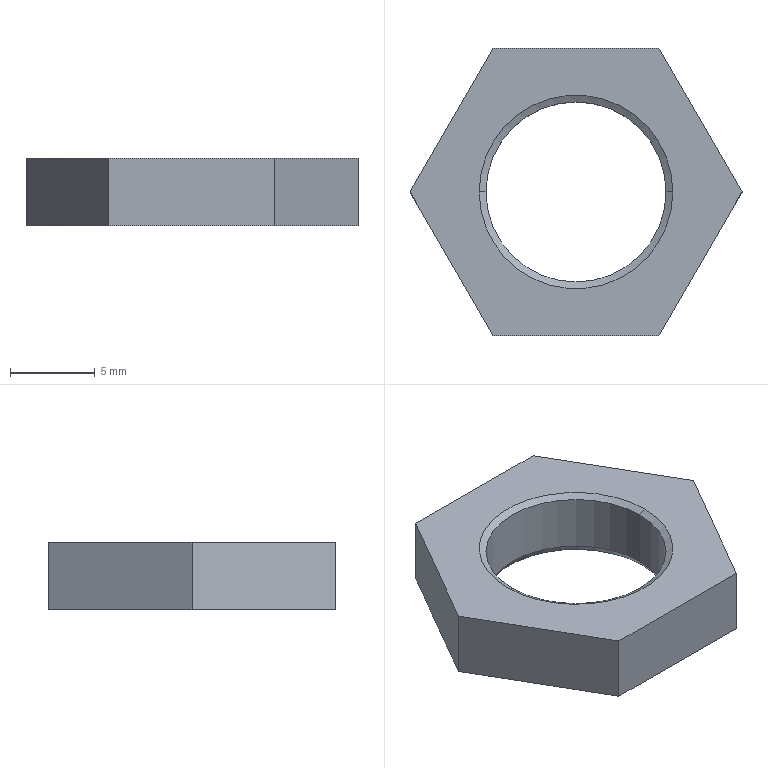Part | STEP file | Fine-Thread Nut M12X1_GB_FASTENER_NUT_STNABTT M12X1.25-N | 1 solid | 14 faces | box 19.63 x 17 x 4 mm | volume 641.848 mm3 | plane 8 | cone 4 | cylinder 2 | commonest cylinder face diameters 10.647 x2
STEP:
#1=CARTESIAN_POINT('',(0.,0.,0.));
#2=DIRECTION('',(0.,0.,1.));
#3=DIRECTION('',(1.,0.,0.));
#4=AXIS2_PLACEMENT_3D('',#1,#2,#3);
#5=CARTESIAN_POINT('',(5.324,0.,-0.2309));
#6=VERTEX_POINT('',#5);
#7=CARTESIAN_POINT('',(5.723,0.,0.));
#8=VERTEX_POINT('',#7);
#9=CARTESIAN_POINT('',(5.324,0.,-0.2309));
#10=DIRECTION('',(0.866,0.,0.5));
#11=VECTOR('',#10,1.);
#12=LINE('',#9,#11);
#13=CARTESIAN_POINT('',(0.,0.,-0.2309));
#14=DIRECTION('',(0.,0.,1.));
#15=DIRECTION('',(1.,0.,0.));
#16=AXIS2_PLACEMENT_3D('',#13,#14,#15);
#17=CONICAL_SURFACE('',#16,5.324,1.047);
#18=CARTESIAN_POINT('',(6.283,0.));
#19=DIRECTION('',(0.,1.));
#20=VECTOR('',#19,1.);
#21=LINE('',#18,#20);
#22=(GEOMETRIC_REPRESENTATION_CONTEXT(2)PARAMETRIC_REPRESENTATION_CONTEXT()REPRESENTATION_CONTEXT('',''));
#23=DEFINITIONAL_REPRESENTATION('',(#21),#22);
#24=PCURVE('',#17,#23);
#25=CARTESIAN_POINT('',(0.,0.,-0.2309));
#26=DIRECTION('',(0.,0.,1.));
#27=DIRECTION('',(1.,0.,0.));
#28=AXIS2_PLACEMENT_3D('',#25,#26,#27);
#29=CONICAL_SURFACE('',#28,5.324,1.047);
#30=CARTESIAN_POINT('',(0.,0.));
#31=DIRECTION('',(0.,1.));
#32=VECTOR('',#31,1.);
#33=LINE('',#30,#32);
#34=(GEOMETRIC_REPRESENTATION_CONTEXT(2)PARAMETRIC_REPRESENTATION_CONTEXT()REPRESENTATION_CONTEXT('',''));
#35=DEFINITIONAL_REPRESENTATION('',(#33),#34);
#36=PCURVE('',#29,#35);
#37=SURFACE_CURVE('',#12,(#24,#36),.PCURVE_S1.);
#38=EDGE_CURVE('',#6,#8,#37,.T.);
#39=ORIENTED_EDGE('',*,*,#38,.T.);
#40=CARTESIAN_POINT('',(-5.723,0.,0.));
#41=VERTEX_POINT('',#40);
#42=CARTESIAN_POINT('',(0.,0.,0.));
#43=DIRECTION('',(0.,0.,-1.));
#44=DIRECTION('',(1.,0.,0.));
#45=AXIS2_PLACEMENT_3D('',#42,#43,#44);
#46=CIRCLE('',#45,5.723);
#47=CARTESIAN_POINT('',(6.283,0.2309));
#48=DIRECTION('',(-1.,0.));
#49=VECTOR('',#48,1.);
#50=LINE('',#47,#49);
#51=(GEOMETRIC_REPRESENTATION_CONTEXT(2)PARAMETRIC_REPRESENTATION_CONTEXT()REPRESENTATION_CONTEXT('',''));
#52=DEFINITIONAL_REPRESENTATION('',(#50),#51);
#53=PCURVE('',#17,#52);
#54=CARTESIAN_POINT('',(4.907,-8.5,0.));
#55=DIRECTION('',(0.,0.,1.));
#56=DIRECTION('',(1.,0.,0.));
#57=AXIS2_PLACEMENT_3D('',#54,#55,#56);
#58=PLANE('',#57);
#59=CARTESIAN_POINT('',(0.816,8.5));
#60=CARTESIAN_POINT('',(0.816,-1.413));
#61=CARTESIAN_POINT('',(-7.769,3.543));
#62=CARTESIAN_POINT('',(-16.354,8.5));
#63=CARTESIAN_POINT('',(-7.769,13.457));
#64=CARTESIAN_POINT('',(0.816,18.413));
#65=CARTESIAN_POINT('',(0.816,8.5));
#66=(BOUNDED_CURVE()B_SPLINE_CURVE(2,(#59,#60,#61,#62,#63,#64,#65),.UNSPECIFIED.,.T.,.F.)B_SPLINE_CURVE_WITH_KNOTS((1,2,2,2,2,1),(-2.094,0.,2.094,4.189,6.283,8.378),.UNSPECIFIED.)CURVE()GEOMETRIC_REPRESENTATION_ITEM()RATIONAL_B_SPLINE_CURVE((1.,0.5,1.,0.5,1.,0.5,1.))REPRESENTATION_ITEM(''));
#67=(GEOMETRIC_REPRESENTATION_CONTEXT(2)PARAMETRIC_REPRESENTATION_CONTEXT()REPRESENTATION_CONTEXT('',''));
#68=DEFINITIONAL_REPRESENTATION('',(#66),#67);
#69=PCURVE('',#58,#68);
#70=SURFACE_CURVE('',#46,(#53,#69),.PCURVE_S1.);
#71=EDGE_CURVE('',#8,#41,#70,.T.);
#72=ORIENTED_EDGE('',*,*,#71,.T.);
#73=CARTESIAN_POINT('',(-5.324,0.,-0.2309));
#74=VERTEX_POINT('',#73);
#75=CARTESIAN_POINT('',(-5.324,0.,-0.2309));
#76=DIRECTION('',(-0.866,0.,0.5));
#77=VECTOR('',#76,1.);
#78=LINE('',#75,#77);
#79=CARTESIAN_POINT('',(3.142,0.));
#80=DIRECTION('',(0.,1.));
#81=VECTOR('',#80,1.);
#82=LINE('',#79,#81);
#83=(GEOMETRIC_REPRESENTATION_CONTEXT(2)PARAMETRIC_REPRESENTATION_CONTEXT()REPRESENTATION_CONTEXT('',''));
#84=DEFINITIONAL_REPRESENTATION('',(#82),#83);
#85=PCURVE('',#17,#84);
#86=CARTESIAN_POINT('',(3.142,0.));
#87=DIRECTION('',(0.,1.));
#88=VECTOR('',#87,1.);
#89=LINE('',#86,#88);
#90=(GEOMETRIC_REPRESENTATION_CONTEXT(2)PARAMETRIC_REPRESENTATION_CONTEXT()REPRESENTATION_CONTEXT('',''));
#91=DEFINITIONAL_REPRESENTATION('',(#89),#90);
#92=PCURVE('',#29,#91);
#93=SURFACE_CURVE('',#78,(#85,#92),.PCURVE_S1.);
#94=EDGE_CURVE('',#74,#41,#93,.T.);
#95=ORIENTED_EDGE('',*,*,#94,.F.);
#96=CARTESIAN_POINT('',(0.,0.,-0.2309));
#97=DIRECTION('',(0.,0.,1.));
#98=DIRECTION('',(1.,0.,0.));
#99=AXIS2_PLACEMENT_3D('',#96,#97,#98);
#100=CIRCLE('',#99,5.324);
#101=CARTESIAN_POINT('',(0.,0.));
#102=DIRECTION('',(1.,0.));
#103=VECTOR('',#102,1.);
#104=LINE('',#101,#103);
#105=(GEOMETRIC_REPRESENTATION_CONTEXT(2)PARAMETRIC_REPRESENTATION_CONTEXT()REPRESENTATION_CONTEXT('',''));
#106=DEFINITIONAL_REPRESENTATION('',(#104),#105);
#107=PCURVE('',#17,#106);
#108=CARTESIAN_POINT('',(0.,0.,-4.));
#109=DIRECTION('',(0.,0.,1.));
#110=DIRECTION('',(1.,0.,0.));
#111=AXIS2_PLACEMENT_3D('',#108,#109,#110);
#112=CYLINDRICAL_SURFACE('',#111,5.324);
#113=CARTESIAN_POINT('',(0.,3.769));
#114=DIRECTION('',(1.,0.));
#115=VECTOR('',#114,1.);
#116=LINE('',#113,#115);
#117=(GEOMETRIC_REPRESENTATION_CONTEXT(2)PARAMETRIC_REPRESENTATION_CONTEXT()REPRESENTATION_CONTEXT('',''));
#118=DEFINITIONAL_REPRESENTATION('',(#116),#117);
#119=PCURVE('',#112,#118);
#120=SURFACE_CURVE('',#100,(#107,#119),.PCURVE_S1.);
#121=EDGE_CURVE('',#74,#6,#120,.T.);
#122=ORIENTED_EDGE('',*,*,#121,.T.);
#123=EDGE_LOOP('',(#39,#72,#95,#122));
#124=FACE_BOUND('',#123,.F.);
#125=ADVANCED_FACE('',(#124),#17,.F.);
#126=CARTESIAN_POINT('',(-5.324,0.,-3.6));
#127=VERTEX_POINT('',#126);
#128=CARTESIAN_POINT('',(-5.554,0.,-4.));
#129=VERTEX_POINT('',#128);
#130=CARTESIAN_POINT('',(-5.554,0.,-4.));
#131=DIRECTION('',(-0.5,0.,-0.866));
#132=VECTOR('',#131,1.);
#133=LINE('',#130,#132);
#134=CARTESIAN_POINT('',(0.,0.,-4.));
#135=DIRECTION('',(0.,0.,-1.));
#136=DIRECTION('',(-1.,0.,0.));
#137=AXIS2_PLACEMENT_3D('',#134,#135,#136);
#138=CONICAL_SURFACE('',#137,5.554,0.5236);
#139=CARTESIAN_POINT('',(6.283,0.));
#140=DIRECTION('',(0.,1.));
#141=VECTOR('',#140,1.);
#142=LINE('',#139,#141);
#143=(GEOMETRIC_REPRESENTATION_CONTEXT(2)PARAMETRIC_REPRESENTATION_CONTEXT()REPRESENTATION_CONTEXT('',''));
#144=DEFINITIONAL_REPRESENTATION('',(#142),#143);
#145=PCURVE('',#138,#144);
#146=CARTESIAN_POINT('',(0.,0.,-4.));
#147=DIRECTION('',(0.,0.,-1.));
#148=DIRECTION('',(-1.,0.,0.));
#149=AXIS2_PLACEMENT_3D('',#146,#147,#148);
#150=CONICAL_SURFACE('',#149,5.554,0.5236);
#151=CARTESIAN_POINT('',(0.,0.));
#152=DIRECTION('',(0.,1.));
#153=VECTOR('',#152,1.);
#154=LINE('',#151,#153);
#155=(GEOMETRIC_REPRESENTATION_CONTEXT(2)PARAMETRIC_REPRESENTATION_CONTEXT()REPRESENTATION_CONTEXT('',''));
#156=DEFINITIONAL_REPRESENTATION('',(#154),#155);
#157=PCURVE('',#150,#156);
#158=SURFACE_CURVE('',#133,(#145,#157),.PCURVE_S1.);
#159=EDGE_CURVE('',#127,#129,#158,.T.);
#160=ORIENTED_EDGE('',*,*,#159,.T.);
#161=CARTESIAN_POINT('',(5.554,0.,-4.));
#162=VERTEX_POINT('',#161);
#163=CARTESIAN_POINT('',(0.,0.,-4.));
#164=DIRECTION('',(0.,0.,1.));
#165=DIRECTION('',(1.,0.,0.));
#166=AXIS2_PLACEMENT_3D('',#163,#164,#165);
#167=CIRCLE('',#166,5.554);
#168=CARTESIAN_POINT('',(9.425,0.));
#169=DIRECTION('',(-1.,0.));
#170=VECTOR('',#169,1.);
#171=LINE('',#168,#170);
#172=(GEOMETRIC_REPRESENTATION_CONTEXT(2)PARAMETRIC_REPRESENTATION_CONTEXT()REPRESENTATION_CONTEXT('',''));
#173=DEFINITIONAL_REPRESENTATION('',(#171),#172);
#174=PCURVE('',#138,#173);
#175=CARTESIAN_POINT('',(4.907,-8.5,-4.));
#176=DIRECTION('',(0.,0.,1.));
#177=DIRECTION('',(1.,0.,0.));
#178=AXIS2_PLACEMENT_3D('',#175,#176,#177);
#179=PLANE('',#178);
#180=CARTESIAN_POINT('',(-4.907,8.5));
#181=DIRECTION('',(1.,0.));
#182=AXIS2_PLACEMENT_2D('',#180,#181);
#183=CIRCLE('',#182,5.554);
#184=(GEOMETRIC_REPRESENTATION_CONTEXT(2)PARAMETRIC_REPRESENTATION_CONTEXT()REPRESENTATION_CONTEXT('',''));
#185=DEFINITIONAL_REPRESENTATION('',(#183),#184);
#186=PCURVE('',#179,#185);
#187=SURFACE_CURVE('',#167,(#174,#186),.PCURVE_S1.);
#188=EDGE_CURVE('',#129,#162,#187,.T.);
#189=ORIENTED_EDGE('',*,*,#188,.T.);
#190=CARTESIAN_POINT('',(5.324,0.,-3.6));
#191=VERTEX_POINT('',#190);
#192=CARTESIAN_POINT('',(5.554,0.,-4.));
#193=DIRECTION('',(0.5,0.,-0.866));
#194=VECTOR('',#193,1.);
#195=LINE('',#192,#194);
#196=CARTESIAN_POINT('',(3.142,0.));
#197=DIRECTION('',(0.,1.));
#198=VECTOR('',#197,1.);
#199=LINE('',#196,#198);
#200=(GEOMETRIC_REPRESENTATION_CONTEXT(2)PARAMETRIC_REPRESENTATION_CONTEXT()REPRESENTATION_CONTEXT('',''));
#201=DEFINITIONAL_REPRESENTATION('',(#199),#200);
#202=PCURVE('',#138,#201);
#203=CARTESIAN_POINT('',(3.142,0.));
#204=DIRECTION('',(0.,1.));
#205=VECTOR('',#204,1.);
#206=LINE('',#203,#205);
#207=(GEOMETRIC_REPRESENTATION_CONTEXT(2)PARAMETRIC_REPRESENTATION_CONTEXT()REPRESENTATION_CONTEXT('',''));
#208=DEFINITIONAL_REPRESENTATION('',(#206),#207);
#209=PCURVE('',#150,#208);
#210=SURFACE_CURVE('',#195,(#202,#209),.PCURVE_S1.);
#211=EDGE_CURVE('',#191,#162,#210,.T.);
#212=ORIENTED_EDGE('',*,*,#211,.F.);
#213=CARTESIAN_POINT('',(0.,0.,-3.6));
#214=DIRECTION('',(0.,0.,-1.));
#215=DIRECTION('',(1.,0.,0.));
#216=AXIS2_PLACEMENT_3D('',#213,#214,#215);
#217=CIRCLE('',#216,5.324);
#218=CARTESIAN_POINT('',(3.142,-0.4));
#219=DIRECTION('',(1.,0.));
#220=VECTOR('',#219,1.);
#221=LINE('',#218,#220);
#222=(GEOMETRIC_REPRESENTATION_CONTEXT(2)PARAMETRIC_REPRESENTATION_CONTEXT()REPRESENTATION_CONTEXT('',''));
#223=DEFINITIONAL_REPRESENTATION('',(#221),#222);
#224=PCURVE('',#138,#223);
#225=CARTESIAN_POINT('',(6.283,0.4));
#226=DIRECTION('',(-1.,0.));
#227=VECTOR('',#226,1.);
#228=LINE('',#225,#227);
#229=(GEOMETRIC_REPRESENTATION_CONTEXT(2)PARAMETRIC_REPRESENTATION_CONTEXT()REPRESENTATION_CONTEXT('',''));
#230=DEFINITIONAL_REPRESENTATION('',(#228),#229);
#231=PCURVE('',#112,#230);
#232=SURFACE_CURVE('',#217,(#224,#231),.PCURVE_S1.);
#233=EDGE_CURVE('',#191,#127,#232,.T.);
#234=ORIENTED_EDGE('',*,*,#233,.T.);
#235=EDGE_LOOP('',(#160,#189,#212,#234));
#236=FACE_BOUND('',#235,.F.);
#237=ADVANCED_FACE('',(#236),#138,.F.);
#238=CARTESIAN_POINT('',(5.324,0.,-4.));
#239=DIRECTION('',(0.,0.,1.));
#240=VECTOR('',#239,1.);
#241=LINE('',#238,#240);
#242=CARTESIAN_POINT('',(6.283,0.));
#243=DIRECTION('',(0.,1.));
#244=VECTOR('',#243,1.);
#245=LINE('',#242,#244);
#246=(GEOMETRIC_REPRESENTATION_CONTEXT(2)PARAMETRIC_REPRESENTATION_CONTEXT()REPRESENTATION_CONTEXT('',''));
#247=DEFINITIONAL_REPRESENTATION('',(#245),#246);
#248=PCURVE('',#112,#247);
#249=CARTESIAN_POINT('',(0.,0.,-4.));
#250=DIRECTION('',(0.,0.,1.));
#251=DIRECTION('',(1.,0.,0.));
#252=AXIS2_PLACEMENT_3D('',#249,#250,#251);
#253=CYLINDRICAL_SURFACE('',#252,5.324);
#254=CARTESIAN_POINT('',(0.,0.));
#255=DIRECTION('',(0.,1.));
#256=VECTOR('',#255,1.);
#257=LINE('',#254,#256);
#258=(GEOMETRIC_REPRESENTATION_CONTEXT(2)PARAMETRIC_REPRESENTATION_CONTEXT()REPRESENTATION_CONTEXT('',''));
#259=DEFINITIONAL_REPRESENTATION('',(#257),#258);
#260=PCURVE('',#253,#259);
#261=SURFACE_CURVE('',#241,(#248,#260),.PCURVE_S1.);
#262=EDGE_CURVE('',#191,#6,#261,.T.);
#263=ORIENTED_EDGE('',*,*,#262,.T.);
#264=ORIENTED_EDGE('',*,*,#121,.F.);
#265=CARTESIAN_POINT('',(-5.324,0.,-4.));
#266=DIRECTION('',(0.,0.,1.));
#267=VECTOR('',#266,1.);
#268=LINE('',#265,#267);
#269=CARTESIAN_POINT('',(3.142,0.));
#270=DIRECTION('',(0.,1.));
#271=VECTOR('',#270,1.);
#272=LINE('',#269,#271);
#273=(GEOMETRIC_REPRESENTATION_CONTEXT(2)PARAMETRIC_REPRESENTATION_CONTEXT()REPRESENTATION_CONTEXT('',''));
#274=DEFINITIONAL_REPRESENTATION('',(#272),#273);
#275=PCURVE('',#112,#274);
#276=CARTESIAN_POINT('',(3.142,0.));
#277=DIRECTION('',(0.,1.));
#278=VECTOR('',#277,1.);
#279=LINE('',#276,#278);
#280=(GEOMETRIC_REPRESENTATION_CONTEXT(2)PARAMETRIC_REPRESENTATION_CONTEXT()REPRESENTATION_CONTEXT('',''));
#281=DEFINITIONAL_REPRESENTATION('',(#279),#280);
#282=PCURVE('',#253,#281);
#283=SURFACE_CURVE('',#268,(#275,#282),.PCURVE_S1.);
#284=EDGE_CURVE('',#127,#74,#283,.T.);
#285=ORIENTED_EDGE('',*,*,#284,.F.);
#286=ORIENTED_EDGE('',*,*,#233,.F.);
#287=EDGE_LOOP('',(#263,#264,#285,#286));
#288=FACE_BOUND('',#287,.F.);
#289=ADVANCED_FACE('',(#288),#112,.F.);
#290=CARTESIAN_POINT('',(-4.907,-8.5,0.));
#291=VERTEX_POINT('',#290);
#292=CARTESIAN_POINT('',(4.907,-8.5,0.));
#293=VERTEX_POINT('',#292);
#294=CARTESIAN_POINT('',(-4.907,-8.5,0.));
#295=DIRECTION('',(1.,0.,0.));
#296=VECTOR('',#295,1.);
#297=LINE('',#294,#296);
#298=CARTESIAN_POINT('',(-4.907,-8.5,-4.));
#299=DIRECTION('',(0.,-1.,0.));
#300=DIRECTION('',(1.,0.,0.));
#301=AXIS2_PLACEMENT_3D('',#298,#299,#300);
#302=PLANE('',#301);
#303=CARTESIAN_POINT('',(0.,4.));
#304=DIRECTION('',(1.,0.));
#305=VECTOR('',#304,1.);
#306=LINE('',#303,#305);
#307=(GEOMETRIC_REPRESENTATION_CONTEXT(2)PARAMETRIC_REPRESENTATION_CONTEXT()REPRESENTATION_CONTEXT('',''));
#308=DEFINITIONAL_REPRESENTATION('',(#306),#307);
#309=PCURVE('',#302,#308);
#310=CARTESIAN_POINT('',(-9.815,0.));
#311=DIRECTION('',(1.,0.));
#312=VECTOR('',#311,1.);
#313=LINE('',#310,#312);
#314=(GEOMETRIC_REPRESENTATION_CONTEXT(2)PARAMETRIC_REPRESENTATION_CONTEXT()REPRESENTATION_CONTEXT('',''));
#315=DEFINITIONAL_REPRESENTATION('',(#313),#314);
#316=PCURVE('',#58,#315);
#317=SURFACE_CURVE('',#297,(#309,#316),.PCURVE_S1.);
#318=EDGE_CURVE('',#291,#293,#317,.T.);
#319=ORIENTED_EDGE('',*,*,#318,.F.);
#320=CARTESIAN_POINT('',(-4.907,-8.5,-4.));
#321=VERTEX_POINT('',#320);
#322=CARTESIAN_POINT('',(-4.907,-8.5,-4.));
#323=DIRECTION('',(0.,0.,1.));
#324=VECTOR('',#323,1.);
#325=LINE('',#322,#324);
#326=CARTESIAN_POINT('',(0.,0.));
#327=DIRECTION('',(0.,1.));
#328=VECTOR('',#327,1.);
#329=LINE('',#326,#328);
#330=(GEOMETRIC_REPRESENTATION_CONTEXT(2)PARAMETRIC_REPRESENTATION_CONTEXT()REPRESENTATION_CONTEXT('',''));
#331=DEFINITIONAL_REPRESENTATION('',(#329),#330);
#332=PCURVE('',#302,#331);
#333=CARTESIAN_POINT('',(-9.815,0.,-4.));
#334=DIRECTION('',(-0.866,-0.5,0.));
#335=DIRECTION('',(0.5,-0.866,0.));
#336=AXIS2_PLACEMENT_3D('',#333,#334,#335);
#337=PLANE('',#336);
#338=CARTESIAN_POINT('',(9.815,0.));
#339=DIRECTION('',(0.,1.));
#340=VECTOR('',#339,1.);
#341=LINE('',#338,#340);
#342=(GEOMETRIC_REPRESENTATION_CONTEXT(2)PARAMETRIC_REPRESENTATION_CONTEXT()REPRESENTATION_CONTEXT('',''));
#343=DEFINITIONAL_REPRESENTATION('',(#341),#342);
#344=PCURVE('',#337,#343);
#345=SURFACE_CURVE('',#325,(#332,#344),.PCURVE_S1.);
#346=EDGE_CURVE('',#321,#291,#345,.T.);
#347=ORIENTED_EDGE('',*,*,#346,.F.);
#348=CARTESIAN_POINT('',(4.907,-8.5,-4.));
#349=VERTEX_POINT('',#348);
#350=CARTESIAN_POINT('',(-4.907,-8.5,-4.));
#351=DIRECTION('',(1.,0.,0.));
#352=VECTOR('',#351,1.);
#353=LINE('',#350,#352);
#354=CARTESIAN_POINT('',(0.,0.));
#355=DIRECTION('',(1.,0.));
#356=VECTOR('',#355,1.);
#357=LINE('',#354,#356);
#358=(GEOMETRIC_REPRESENTATION_CONTEXT(2)PARAMETRIC_REPRESENTATION_CONTEXT()REPRESENTATION_CONTEXT('',''));
#359=DEFINITIONAL_REPRESENTATION('',(#357),#358);
#360=PCURVE('',#302,#359);
#361=CARTESIAN_POINT('',(-9.815,0.));
#362=DIRECTION('',(1.,0.));
#363=VECTOR('',#362,1.);
#364=LINE('',#361,#363);
#365=(GEOMETRIC_REPRESENTATION_CONTEXT(2)PARAMETRIC_REPRESENTATION_CONTEXT()REPRESENTATION_CONTEXT('',''));
#366=DEFINITIONAL_REPRESENTATION('',(#364),#365);
#367=PCURVE('',#179,#366);
#368=SURFACE_CURVE('',#353,(#360,#367),.PCURVE_S1.);
#369=EDGE_CURVE('',#321,#349,#368,.T.);
#370=ORIENTED_EDGE('',*,*,#369,.T.);
#371=CARTESIAN_POINT('',(4.907,-8.5,-4.));
#372=DIRECTION('',(0.,0.,1.));
#373=VECTOR('',#372,1.);
#374=LINE('',#371,#373);
#375=CARTESIAN_POINT('',(9.815,0.));
#376=DIRECTION('',(0.,1.));
#377=VECTOR('',#376,1.);
#378=LINE('',#375,#377);
#379=(GEOMETRIC_REPRESENTATION_CONTEXT(2)PARAMETRIC_REPRESENTATION_CONTEXT()REPRESENTATION_CONTEXT('',''));
#380=DEFINITIONAL_REPRESENTATION('',(#378),#379);
#381=PCURVE('',#302,#380);
#382=CARTESIAN_POINT('',(4.907,-8.5,-4.));
#383=DIRECTION('',(0.866,-0.5,0.));
#384=DIRECTION('',(0.5,0.866,0.));
#385=AXIS2_PLACEMENT_3D('',#382,#383,#384);
#386=PLANE('',#385);
#387=CARTESIAN_POINT('',(0.,0.));
#388=DIRECTION('',(0.,1.));
#389=VECTOR('',#388,1.);
#390=LINE('',#387,#389);
#391=(GEOMETRIC_REPRESENTATION_CONTEXT(2)PARAMETRIC_REPRESENTATION_CONTEXT()REPRESENTATION_CONTEXT('',''));
#392=DEFINITIONAL_REPRESENTATION('',(#390),#391);
#393=PCURVE('',#386,#392);
#394=SURFACE_CURVE('',#374,(#381,#393),.PCURVE_S1.);
#395=EDGE_CURVE('',#349,#293,#394,.T.);
#396=ORIENTED_EDGE('',*,*,#395,.T.);
#397=EDGE_LOOP('',(#319,#347,#370,#396));
#398=FACE_BOUND('',#397,.T.);
#399=ADVANCED_FACE('',(#398),#302,.T.);
#400=CARTESIAN_POINT('',(-9.815,0.,0.));
#401=VERTEX_POINT('',#400);
#402=CARTESIAN_POINT('',(-9.815,0.,0.));
#403=DIRECTION('',(0.5,-0.866,0.));
#404=VECTOR('',#403,1.);
#405=LINE('',#402,#404);
#406=CARTESIAN_POINT('',(0.,4.));
#407=DIRECTION('',(1.,0.));
#408=VECTOR('',#407,1.);
#409=LINE('',#406,#408);
#410=(GEOMETRIC_REPRESENTATION_CONTEXT(2)PARAMETRIC_REPRESENTATION_CONTEXT()REPRESENTATION_CONTEXT('',''));
#411=DEFINITIONAL_REPRESENTATION('',(#409),#410);
#412=PCURVE('',#337,#411);
#413=CARTESIAN_POINT('',(-14.722,8.5));
#414=DIRECTION('',(0.5,-0.866));
#415=VECTOR('',#414,1.);
#416=LINE('',#413,#415);
#417=(GEOMETRIC_REPRESENTATION_CONTEXT(2)PARAMETRIC_REPRESENTATION_CONTEXT()REPRESENTATION_CONTEXT('',''));
#418=DEFINITIONAL_REPRESENTATION('',(#416),#417);
#419=PCURVE('',#58,#418);
#420=SURFACE_CURVE('',#405,(#412,#419),.PCURVE_S1.);
#421=EDGE_CURVE('',#401,#291,#420,.T.);
#422=ORIENTED_EDGE('',*,*,#421,.F.);
#423=CARTESIAN_POINT('',(-9.815,0.,-4.));
#424=VERTEX_POINT('',#423);
#425=CARTESIAN_POINT('',(-9.815,0.,-4.));
#426=DIRECTION('',(0.,0.,1.));
#427=VECTOR('',#426,1.);
#428=LINE('',#425,#427);
#429=CARTESIAN_POINT('',(0.,0.));
#430=DIRECTION('',(0.,1.));
#431=VECTOR('',#430,1.);
#432=LINE('',#429,#431);
#433=(GEOMETRIC_REPRESENTATION_CONTEXT(2)PARAMETRIC_REPRESENTATION_CONTEXT()REPRESENTATION_CONTEXT('',''));
#434=DEFINITIONAL_REPRESENTATION('',(#432),#433);
#435=PCURVE('',#337,#434);
#436=CARTESIAN_POINT('',(-4.907,8.5,-4.));
#437=DIRECTION('',(-0.866,0.5,0.));
#438=DIRECTION('',(-0.5,-0.866,0.));
#439=AXIS2_PLACEMENT_3D('',#436,#437,#438);
#440=PLANE('',#439);
#441=CARTESIAN_POINT('',(9.815,0.));
#442=DIRECTION('',(0.,1.));
#443=VECTOR('',#442,1.);
#444=LINE('',#441,#443);
#445=(GEOMETRIC_REPRESENTATION_CONTEXT(2)PARAMETRIC_REPRESENTATION_CONTEXT()REPRESENTATION_CONTEXT('',''));
#446=DEFINITIONAL_REPRESENTATION('',(#444),#445);
#447=PCURVE('',#440,#446);
#448=SURFACE_CURVE('',#428,(#435,#447),.PCURVE_S1.);
#449=EDGE_CURVE('',#424,#401,#448,.T.);
#450=ORIENTED_EDGE('',*,*,#449,.F.);
#451=CARTESIAN_POINT('',(-9.815,0.,-4.));
#452=DIRECTION('',(0.5,-0.866,0.));
#453=VECTOR('',#452,1.);
#454=LINE('',#451,#453);
#455=CARTESIAN_POINT('',(0.,0.));
#456=DIRECTION('',(1.,0.));
#457=VECTOR('',#456,1.);
#458=LINE('',#455,#457);
#459=(GEOMETRIC_REPRESENTATION_CONTEXT(2)PARAMETRIC_REPRESENTATION_CONTEXT()REPRESENTATION_CONTEXT('',''));
#460=DEFINITIONAL_REPRESENTATION('',(#458),#459);
#461=PCURVE('',#337,#460);
#462=CARTESIAN_POINT('',(-14.722,8.5));
#463=DIRECTION('',(0.5,-0.866));
#464=VECTOR('',#463,1.);
#465=LINE('',#462,#464);
#466=(GEOMETRIC_REPRESENTATION_CONTEXT(2)PARAMETRIC_REPRESENTATION_CONTEXT()REPRESENTATION_CONTEXT('',''));
#467=DEFINITIONAL_REPRESENTATION('',(#465),#466);
#468=PCURVE('',#179,#467);
#469=SURFACE_CURVE('',#454,(#461,#468),.PCURVE_S1.);
#470=EDGE_CURVE('',#424,#321,#469,.T.);
#471=ORIENTED_EDGE('',*,*,#470,.T.);
#472=ORIENTED_EDGE('',*,*,#346,.T.);
#473=EDGE_LOOP('',(#422,#450,#471,#472));
#474=FACE_BOUND('',#473,.T.);
#475=ADVANCED_FACE('',(#474),#337,.T.);
#476=CARTESIAN_POINT('',(-4.907,8.5,0.));
#477=VERTEX_POINT('',#476);
#478=CARTESIAN_POINT('',(-4.907,8.5,0.));
#479=DIRECTION('',(-0.5,-0.866,0.));
#480=VECTOR('',#479,1.);
#481=LINE('',#478,#480);
#482=CARTESIAN_POINT('',(0.,4.));
#483=DIRECTION('',(1.,0.));
#484=VECTOR('',#483,1.);
#485=LINE('',#482,#484);
#486=(GEOMETRIC_REPRESENTATION_CONTEXT(2)PARAMETRIC_REPRESENTATION_CONTEXT()REPRESENTATION_CONTEXT('',''));
#487=DEFINITIONAL_REPRESENTATION('',(#485),#486);
#488=PCURVE('',#440,#487);
#489=CARTESIAN_POINT('',(-9.815,17.));
#490=DIRECTION('',(-0.5,-0.866));
#491=VECTOR('',#490,1.);
#492=LINE('',#489,#491);
#493=(GEOMETRIC_REPRESENTATION_CONTEXT(2)PARAMETRIC_REPRESENTATION_CONTEXT()REPRESENTATION_CONTEXT('',''));
#494=DEFINITIONAL_REPRESENTATION('',(#492),#493);
#495=PCURVE('',#58,#494);
#496=SURFACE_CURVE('',#481,(#488,#495),.PCURVE_S1.);
#497=EDGE_CURVE('',#477,#401,#496,.T.);
#498=ORIENTED_EDGE('',*,*,#497,.F.);
#499=CARTESIAN_POINT('',(-4.907,8.5,-4.));
#500=VERTEX_POINT('',#499);
#501=CARTESIAN_POINT('',(-4.907,8.5,-4.));
#502=DIRECTION('',(0.,0.,1.));
#503=VECTOR('',#502,1.);
#504=LINE('',#501,#503);
#505=CARTESIAN_POINT('',(0.,0.));
#506=DIRECTION('',(0.,1.));
#507=VECTOR('',#506,1.);
#508=LINE('',#505,#507);
#509=(GEOMETRIC_REPRESENTATION_CONTEXT(2)PARAMETRIC_REPRESENTATION_CONTEXT()REPRESENTATION_CONTEXT('',''));
#510=DEFINITIONAL_REPRESENTATION('',(#508),#509);
#511=PCURVE('',#440,#510);
#512=CARTESIAN_POINT('',(4.907,8.5,-4.));
#513=DIRECTION('',(0.,1.,0.));
#514=DIRECTION('',(0.,0.,1.));
#515=AXIS2_PLACEMENT_3D('',#512,#513,#514);
#516=PLANE('',#515);
#517=CARTESIAN_POINT('',(0.,-9.815));
#518=DIRECTION('',(1.,0.));
#519=VECTOR('',#518,1.);
#520=LINE('',#517,#519);
#521=(GEOMETRIC_REPRESENTATION_CONTEXT(2)PARAMETRIC_REPRESENTATION_CONTEXT()REPRESENTATION_CONTEXT('',''));
#522=DEFINITIONAL_REPRESENTATION('',(#520),#521);
#523=PCURVE('',#516,#522);
#524=SURFACE_CURVE('',#504,(#511,#523),.PCURVE_S1.);
#525=EDGE_CURVE('',#500,#477,#524,.T.);
#526=ORIENTED_EDGE('',*,*,#525,.F.);
#527=CARTESIAN_POINT('',(-4.907,8.5,-4.));
#528=DIRECTION('',(-0.5,-0.866,0.));
#529=VECTOR('',#528,1.);
#530=LINE('',#527,#529);
#531=CARTESIAN_POINT('',(0.,0.));
#532=DIRECTION('',(1.,0.));
#533=VECTOR('',#532,1.);
#534=LINE('',#531,#533);
#535=(GEOMETRIC_REPRESENTATION_CONTEXT(2)PARAMETRIC_REPRESENTATION_CONTEXT()REPRESENTATION_CONTEXT('',''));
#536=DEFINITIONAL_REPRESENTATION('',(#534),#535);
#537=PCURVE('',#440,#536);
#538=CARTESIAN_POINT('',(-9.815,17.));
#539=DIRECTION('',(-0.5,-0.866));
#540=VECTOR('',#539,1.);
#541=LINE('',#538,#540);
#542=(GEOMETRIC_REPRESENTATION_CONTEXT(2)PARAMETRIC_REPRESENTATION_CONTEXT()REPRESENTATION_CONTEXT('',''));
#543=DEFINITIONAL_REPRESENTATION('',(#541),#542);
#544=PCURVE('',#179,#543);
#545=SURFACE_CURVE('',#530,(#537,#544),.PCURVE_S1.);
#546=EDGE_CURVE('',#500,#424,#545,.T.);
#547=ORIENTED_EDGE('',*,*,#546,.T.);
#548=ORIENTED_EDGE('',*,*,#449,.T.);
#549=EDGE_LOOP('',(#498,#526,#547,#548));
#550=FACE_BOUND('',#549,.T.);
#551=ADVANCED_FACE('',(#550),#440,.T.);
#552=CARTESIAN_POINT('',(4.907,8.5,0.));
#553=VERTEX_POINT('',#552);
#554=CARTESIAN_POINT('',(4.907,8.5,0.));
#555=DIRECTION('',(-1.,0.,0.));
#556=VECTOR('',#555,1.);
#557=LINE('',#554,#556);
#558=CARTESIAN_POINT('',(4.,0.));
#559=DIRECTION('',(0.,-1.));
#560=VECTOR('',#559,1.);
#561=LINE('',#558,#560);
#562=(GEOMETRIC_REPRESENTATION_CONTEXT(2)PARAMETRIC_REPRESENTATION_CONTEXT()REPRESENTATION_CONTEXT('',''));
#563=DEFINITIONAL_REPRESENTATION('',(#561),#562);
#564=PCURVE('',#516,#563);
#565=CARTESIAN_POINT('',(0.,17.));
#566=DIRECTION('',(-1.,0.));
#567=VECTOR('',#566,1.);
#568=LINE('',#565,#567);
#569=(GEOMETRIC_REPRESENTATION_CONTEXT(2)PARAMETRIC_REPRESENTATION_CONTEXT()REPRESENTATION_CONTEXT('',''));
#570=DEFINITIONAL_REPRESENTATION('',(#568),#569);
#571=PCURVE('',#58,#570);
#572=SURFACE_CURVE('',#557,(#564,#571),.PCURVE_S1.);
#573=EDGE_CURVE('',#553,#477,#572,.T.);
#574=ORIENTED_EDGE('',*,*,#573,.F.);
#575=CARTESIAN_POINT('',(4.907,8.5,-4.));
#576=VERTEX_POINT('',#575);
#577=CARTESIAN_POINT('',(4.907,8.5,-4.));
#578=DIRECTION('',(0.,0.,1.));
#579=VECTOR('',#578,1.);
#580=LINE('',#577,#579);
#581=CARTESIAN_POINT('',(0.,0.));
#582=DIRECTION('',(1.,0.));
#583=VECTOR('',#582,1.);
#584=LINE('',#581,#583);
#585=(GEOMETRIC_REPRESENTATION_CONTEXT(2)PARAMETRIC_REPRESENTATION_CONTEXT()REPRESENTATION_CONTEXT('',''));
#586=DEFINITIONAL_REPRESENTATION('',(#584),#585);
#587=PCURVE('',#516,#586);
#588=CARTESIAN_POINT('',(9.815,0.,-4.));
#589=DIRECTION('',(0.866,0.5,0.));
#590=DIRECTION('',(-0.5,0.866,0.));
#591=AXIS2_PLACEMENT_3D('',#588,#589,#590);
#592=PLANE('',#591);
#593=CARTESIAN_POINT('',(9.815,0.));
#594=DIRECTION('',(0.,1.));
#595=VECTOR('',#594,1.);
#596=LINE('',#593,#595);
#597=(GEOMETRIC_REPRESENTATION_CONTEXT(2)PARAMETRIC_REPRESENTATION_CONTEXT()REPRESENTATION_CONTEXT('',''));
#598=DEFINITIONAL_REPRESENTATION('',(#596),#597);
#599=PCURVE('',#592,#598);
#600=SURFACE_CURVE('',#580,(#587,#599),.PCURVE_S1.);
#601=EDGE_CURVE('',#576,#553,#600,.T.);
#602=ORIENTED_EDGE('',*,*,#601,.F.);
#603=CARTESIAN_POINT('',(4.907,8.5,-4.));
#604=DIRECTION('',(-1.,0.,0.));
#605=VECTOR('',#604,1.);
#606=LINE('',#603,#605);
#607=CARTESIAN_POINT('',(0.,0.));
#608=DIRECTION('',(0.,-1.));
#609=VECTOR('',#608,1.);
#610=LINE('',#607,#609);
#611=(GEOMETRIC_REPRESENTATION_CONTEXT(2)PARAMETRIC_REPRESENTATION_CONTEXT()REPRESENTATION_CONTEXT('',''));
#612=DEFINITIONAL_REPRESENTATION('',(#610),#611);
#613=PCURVE('',#516,#612);
#614=CARTESIAN_POINT('',(0.,17.));
#615=DIRECTION('',(-1.,0.));
#616=VECTOR('',#615,1.);
#617=LINE('',#614,#616);
#618=(GEOMETRIC_REPRESENTATION_CONTEXT(2)PARAMETRIC_REPRESENTATION_CONTEXT()REPRESENTATION_CONTEXT('',''));
#619=DEFINITIONAL_REPRESENTATION('',(#617),#618);
#620=PCURVE('',#179,#619);
#621=SURFACE_CURVE('',#606,(#613,#620),.PCURVE_S1.);
#622=EDGE_CURVE('',#576,#500,#621,.T.);
#623=ORIENTED_EDGE('',*,*,#622,.T.);
#624=ORIENTED_EDGE('',*,*,#525,.T.);
#625=EDGE_LOOP('',(#574,#602,#623,#624));
#626=FACE_BOUND('',#625,.T.);
#627=ADVANCED_FACE('',(#626),#516,.T.);
#628=CARTESIAN_POINT('',(9.815,0.,0.));
#629=VERTEX_POINT('',#628);
#630=CARTESIAN_POINT('',(9.815,0.,0.));
#631=DIRECTION('',(-0.5,0.866,0.));
#632=VECTOR('',#631,1.);
#633=LINE('',#630,#632);
#634=CARTESIAN_POINT('',(0.,4.));
#635=DIRECTION('',(1.,0.));
#636=VECTOR('',#635,1.);
#637=LINE('',#634,#636);
#638=(GEOMETRIC_REPRESENTATION_CONTEXT(2)PARAMETRIC_REPRESENTATION_CONTEXT()REPRESENTATION_CONTEXT('',''));
#639=DEFINITIONAL_REPRESENTATION('',(#637),#638);
#640=PCURVE('',#592,#639);
#641=CARTESIAN_POINT('',(4.907,8.5));
#642=DIRECTION('',(-0.5,0.866));
#643=VECTOR('',#642,1.);
#644=LINE('',#641,#643);
#645=(GEOMETRIC_REPRESENTATION_CONTEXT(2)PARAMETRIC_REPRESENTATION_CONTEXT()REPRESENTATION_CONTEXT('',''));
#646=DEFINITIONAL_REPRESENTATION('',(#644),#645);
#647=PCURVE('',#58,#646);
#648=SURFACE_CURVE('',#633,(#640,#647),.PCURVE_S1.);
#649=EDGE_CURVE('',#629,#553,#648,.T.);
#650=ORIENTED_EDGE('',*,*,#649,.F.);
#651=CARTESIAN_POINT('',(9.815,0.,-4.));
#652=VERTEX_POINT('',#651);
#653=CARTESIAN_POINT('',(9.815,0.,-4.));
#654=DIRECTION('',(0.,0.,1.));
#655=VECTOR('',#654,1.);
#656=LINE('',#653,#655);
#657=CARTESIAN_POINT('',(0.,0.));
#658=DIRECTION('',(0.,1.));
#659=VECTOR('',#658,1.);
#660=LINE('',#657,#659);
#661=(GEOMETRIC_REPRESENTATION_CONTEXT(2)PARAMETRIC_REPRESENTATION_CONTEXT()REPRESENTATION_CONTEXT('',''));
#662=DEFINITIONAL_REPRESENTATION('',(#660),#661);
#663=PCURVE('',#592,#662);
#664=CARTESIAN_POINT('',(9.815,0.));
#665=DIRECTION('',(0.,1.));
#666=VECTOR('',#665,1.);
#667=LINE('',#664,#666);
#668=(GEOMETRIC_REPRESENTATION_CONTEXT(2)PARAMETRIC_REPRESENTATION_CONTEXT()REPRESENTATION_CONTEXT('',''));
#669=DEFINITIONAL_REPRESENTATION('',(#667),#668);
#670=PCURVE('',#386,#669);
#671=SURFACE_CURVE('',#656,(#663,#670),.PCURVE_S1.);
#672=EDGE_CURVE('',#652,#629,#671,.T.);
#673=ORIENTED_EDGE('',*,*,#672,.F.);
#674=CARTESIAN_POINT('',(9.815,0.,-4.));
#675=DIRECTION('',(-0.5,0.866,0.));
#676=VECTOR('',#675,1.);
#677=LINE('',#674,#676);
#678=CARTESIAN_POINT('',(0.,0.));
#679=DIRECTION('',(1.,0.));
#680=VECTOR('',#679,1.);
#681=LINE('',#678,#680);
#682=(GEOMETRIC_REPRESENTATION_CONTEXT(2)PARAMETRIC_REPRESENTATION_CONTEXT()REPRESENTATION_CONTEXT('',''));
#683=DEFINITIONAL_REPRESENTATION('',(#681),#682);
#684=PCURVE('',#592,#683);
#685=CARTESIAN_POINT('',(4.907,8.5));
#686=DIRECTION('',(-0.5,0.866));
#687=VECTOR('',#686,1.);
#688=LINE('',#685,#687);
#689=(GEOMETRIC_REPRESENTATION_CONTEXT(2)PARAMETRIC_REPRESENTATION_CONTEXT()REPRESENTATION_CONTEXT('',''));
#690=DEFINITIONAL_REPRESENTATION('',(#688),#689);
#691=PCURVE('',#179,#690);
#692=SURFACE_CURVE('',#677,(#684,#691),.PCURVE_S1.);
#693=EDGE_CURVE('',#652,#576,#692,.T.);
#694=ORIENTED_EDGE('',*,*,#693,.T.);
#695=ORIENTED_EDGE('',*,*,#601,.T.);
#696=EDGE_LOOP('',(#650,#673,#694,#695));
#697=FACE_BOUND('',#696,.T.);
#698=ADVANCED_FACE('',(#697),#592,.T.);
#699=CARTESIAN_POINT('',(4.907,-8.5,0.));
#700=DIRECTION('',(0.5,0.866,0.));
#701=VECTOR('',#700,1.);
#702=LINE('',#699,#701);
#703=CARTESIAN_POINT('',(0.,4.));
#704=DIRECTION('',(1.,0.));
#705=VECTOR('',#704,1.);
#706=LINE('',#703,#705);
#707=(GEOMETRIC_REPRESENTATION_CONTEXT(2)PARAMETRIC_REPRESENTATION_CONTEXT()REPRESENTATION_CONTEXT('',''));
#708=DEFINITIONAL_REPRESENTATION('',(#706),#707);
#709=PCURVE('',#386,#708);
#710=CARTESIAN_POINT('',(0.,0.));
#711=DIRECTION('',(0.5,0.866));
#712=VECTOR('',#711,1.);
#713=LINE('',#710,#712);
#714=(GEOMETRIC_REPRESENTATION_CONTEXT(2)PARAMETRIC_REPRESENTATION_CONTEXT()REPRESENTATION_CONTEXT('',''));
#715=DEFINITIONAL_REPRESENTATION('',(#713),#714);
#716=PCURVE('',#58,#715);
#717=SURFACE_CURVE('',#702,(#709,#716),.PCURVE_S1.);
#718=EDGE_CURVE('',#293,#629,#717,.T.);
#719=ORIENTED_EDGE('',*,*,#718,.F.);
#720=ORIENTED_EDGE('',*,*,#395,.F.);
#721=CARTESIAN_POINT('',(4.907,-8.5,-4.));
#722=DIRECTION('',(0.5,0.866,0.));
#723=VECTOR('',#722,1.);
#724=LINE('',#721,#723);
#725=CARTESIAN_POINT('',(0.,0.));
#726=DIRECTION('',(1.,0.));
#727=VECTOR('',#726,1.);
#728=LINE('',#725,#727);
#729=(GEOMETRIC_REPRESENTATION_CONTEXT(2)PARAMETRIC_REPRESENTATION_CONTEXT()REPRESENTATION_CONTEXT('',''));
#730=DEFINITIONAL_REPRESENTATION('',(#728),#729);
#731=PCURVE('',#386,#730);
#732=CARTESIAN_POINT('',(0.,0.));
#733=DIRECTION('',(0.5,0.866));
#734=VECTOR('',#733,1.);
#735=LINE('',#732,#734);
#736=(GEOMETRIC_REPRESENTATION_CONTEXT(2)PARAMETRIC_REPRESENTATION_CONTEXT()REPRESENTATION_CONTEXT('',''));
#737=DEFINITIONAL_REPRESENTATION('',(#735),#736);
#738=PCURVE('',#179,#737);
#739=SURFACE_CURVE('',#724,(#731,#738),.PCURVE_S1.);
#740=EDGE_CURVE('',#349,#652,#739,.T.);
#741=ORIENTED_EDGE('',*,*,#740,.T.);
#742=ORIENTED_EDGE('',*,*,#672,.T.);
#743=EDGE_LOOP('',(#719,#720,#741,#742));
#744=FACE_BOUND('',#743,.T.);
#745=ADVANCED_FACE('',(#744),#386,.T.);
#746=ORIENTED_EDGE('',*,*,#188,.T.);
#747=CARTESIAN_POINT('',(0.,0.,-4.));
#748=DIRECTION('',(0.,0.,1.));
#749=DIRECTION('',(1.,0.,0.));
#750=AXIS2_PLACEMENT_3D('',#747,#748,#749);
#751=CIRCLE('',#750,5.554);
#752=CARTESIAN_POINT('',(-4.907,8.5));
#753=DIRECTION('',(1.,0.));
#754=AXIS2_PLACEMENT_2D('',#752,#753);
#755=CIRCLE('',#754,5.554);
#756=(GEOMETRIC_REPRESENTATION_CONTEXT(2)PARAMETRIC_REPRESENTATION_CONTEXT()REPRESENTATION_CONTEXT('',''));
#757=DEFINITIONAL_REPRESENTATION('',(#755),#756);
#758=PCURVE('',#179,#757);
#759=CARTESIAN_POINT('',(3.142,0.));
#760=DIRECTION('',(-1.,0.));
#761=VECTOR('',#760,1.);
#762=LINE('',#759,#761);
#763=(GEOMETRIC_REPRESENTATION_CONTEXT(2)PARAMETRIC_REPRESENTATION_CONTEXT()REPRESENTATION_CONTEXT('',''));
#764=DEFINITIONAL_REPRESENTATION('',(#762),#763);
#765=PCURVE('',#150,#764);
#766=SURFACE_CURVE('',#751,(#758,#765),.PCURVE_S1.);
#767=EDGE_CURVE('',#162,#129,#766,.T.);
#768=ORIENTED_EDGE('',*,*,#767,.T.);
#769=EDGE_LOOP('',(#746,#768));
#770=FACE_BOUND('',#769,.T.);
#771=ORIENTED_EDGE('',*,*,#369,.F.);
#772=ORIENTED_EDGE('',*,*,#470,.F.);
#773=ORIENTED_EDGE('',*,*,#546,.F.);
#774=ORIENTED_EDGE('',*,*,#622,.F.);
#775=ORIENTED_EDGE('',*,*,#693,.F.);
#776=ORIENTED_EDGE('',*,*,#740,.F.);
#777=EDGE_LOOP('',(#771,#772,#773,#774,#775,#776));
#778=FACE_BOUND('',#777,.T.);
#779=ADVANCED_FACE('',(#770,#778),#179,.F.);
#780=ORIENTED_EDGE('',*,*,#71,.T.);
#781=CARTESIAN_POINT('',(0.,0.,0.));
#782=DIRECTION('',(0.,0.,-1.));
#783=DIRECTION('',(1.,0.,0.));
#784=AXIS2_PLACEMENT_3D('',#781,#782,#783);
#785=CIRCLE('',#784,5.723);
#786=CARTESIAN_POINT('',(0.816,8.5));
#787=CARTESIAN_POINT('',(0.816,-1.413));
#788=CARTESIAN_POINT('',(-7.769,3.543));
#789=CARTESIAN_POINT('',(-16.354,8.5));
#790=CARTESIAN_POINT('',(-7.769,13.457));
#791=CARTESIAN_POINT('',(0.816,18.413));
#792=CARTESIAN_POINT('',(0.816,8.5));
#793=(BOUNDED_CURVE()B_SPLINE_CURVE(2,(#786,#787,#788,#789,#790,#791,#792),.UNSPECIFIED.,.T.,.F.)B_SPLINE_CURVE_WITH_KNOTS((1,2,2,2,2,1),(-2.094,0.,2.094,4.189,6.283,8.378),.UNSPECIFIED.)CURVE()GEOMETRIC_REPRESENTATION_ITEM()RATIONAL_B_SPLINE_CURVE((1.,0.5,1.,0.5,1.,0.5,1.))REPRESENTATION_ITEM(''));
#794=(GEOMETRIC_REPRESENTATION_CONTEXT(2)PARAMETRIC_REPRESENTATION_CONTEXT()REPRESENTATION_CONTEXT('',''));
#795=DEFINITIONAL_REPRESENTATION('',(#793),#794);
#796=PCURVE('',#58,#795);
#797=CARTESIAN_POINT('',(6.283,0.2309));
#798=DIRECTION('',(-1.,0.));
#799=VECTOR('',#798,1.);
#800=LINE('',#797,#799);
#801=(GEOMETRIC_REPRESENTATION_CONTEXT(2)PARAMETRIC_REPRESENTATION_CONTEXT()REPRESENTATION_CONTEXT('',''));
#802=DEFINITIONAL_REPRESENTATION('',(#800),#801);
#803=PCURVE('',#29,#802);
#804=SURFACE_CURVE('',#785,(#796,#803),.PCURVE_S1.);
#805=EDGE_CURVE('',#41,#8,#804,.T.);
#806=ORIENTED_EDGE('',*,*,#805,.T.);
#807=EDGE_LOOP('',(#780,#806));
#808=FACE_BOUND('',#807,.T.);
#809=ORIENTED_EDGE('',*,*,#318,.T.);
#810=ORIENTED_EDGE('',*,*,#718,.T.);
#811=ORIENTED_EDGE('',*,*,#649,.T.);
#812=ORIENTED_EDGE('',*,*,#573,.T.);
#813=ORIENTED_EDGE('',*,*,#497,.T.);
#814=ORIENTED_EDGE('',*,*,#421,.T.);
#815=EDGE_LOOP('',(#809,#810,#811,#812,#813,#814));
#816=FACE_BOUND('',#815,.T.);
#817=ADVANCED_FACE('',(#808,#816),#58,.T.);
#818=CARTESIAN_POINT('',(0.,0.,-0.2309));
#819=DIRECTION('',(0.,0.,1.));
#820=DIRECTION('',(1.,0.,0.));
#821=AXIS2_PLACEMENT_3D('',#818,#819,#820);
#822=CIRCLE('',#821,5.324);
#823=CARTESIAN_POINT('',(0.,3.769));
#824=DIRECTION('',(1.,0.));
#825=VECTOR('',#824,1.);
#826=LINE('',#823,#825);
#827=(GEOMETRIC_REPRESENTATION_CONTEXT(2)PARAMETRIC_REPRESENTATION_CONTEXT()REPRESENTATION_CONTEXT('',''));
#828=DEFINITIONAL_REPRESENTATION('',(#826),#827);
#829=PCURVE('',#253,#828);
#830=CARTESIAN_POINT('',(0.,0.));
#831=DIRECTION('',(1.,0.));
#832=VECTOR('',#831,1.);
#833=LINE('',#830,#832);
#834=(GEOMETRIC_REPRESENTATION_CONTEXT(2)PARAMETRIC_REPRESENTATION_CONTEXT()REPRESENTATION_CONTEXT('',''));
#835=DEFINITIONAL_REPRESENTATION('',(#833),#834);
#836=PCURVE('',#29,#835);
#837=SURFACE_CURVE('',#822,(#829,#836),.PCURVE_S1.);
#838=EDGE_CURVE('',#6,#74,#837,.T.);
#839=ORIENTED_EDGE('',*,*,#838,.F.);
#840=ORIENTED_EDGE('',*,*,#262,.F.);
#841=CARTESIAN_POINT('',(0.,0.,-3.6));
#842=DIRECTION('',(0.,0.,-1.));
#843=DIRECTION('',(1.,0.,0.));
#844=AXIS2_PLACEMENT_3D('',#841,#842,#843);
#845=CIRCLE('',#844,5.324);
#846=CARTESIAN_POINT('',(6.283,0.4));
#847=DIRECTION('',(-1.,0.));
#848=VECTOR('',#847,1.);
#849=LINE('',#846,#848);
#850=(GEOMETRIC_REPRESENTATION_CONTEXT(2)PARAMETRIC_REPRESENTATION_CONTEXT()REPRESENTATION_CONTEXT('',''));
#851=DEFINITIONAL_REPRESENTATION('',(#849),#850);
#852=PCURVE('',#253,#851);
#853=CARTESIAN_POINT('',(-3.142,-0.4));
#854=DIRECTION('',(1.,0.));
#855=VECTOR('',#854,1.);
#856=LINE('',#853,#855);
#857=(GEOMETRIC_REPRESENTATION_CONTEXT(2)PARAMETRIC_REPRESENTATION_CONTEXT()REPRESENTATION_CONTEXT('',''));
#858=DEFINITIONAL_REPRESENTATION('',(#856),#857);
#859=PCURVE('',#150,#858);
#860=SURFACE_CURVE('',#845,(#852,#859),.PCURVE_S1.);
#861=EDGE_CURVE('',#127,#191,#860,.T.);
#862=ORIENTED_EDGE('',*,*,#861,.F.);
#863=ORIENTED_EDGE('',*,*,#284,.T.);
#864=EDGE_LOOP('',(#839,#840,#862,#863));
#865=FACE_BOUND('',#864,.F.);
#866=ADVANCED_FACE('',(#865),#253,.F.);
#867=ORIENTED_EDGE('',*,*,#767,.T.);
#868=ORIENTED_EDGE('',*,*,#159,.F.);
#869=ORIENTED_EDGE('',*,*,#861,.T.);
#870=ORIENTED_EDGE('',*,*,#211,.T.);
#871=EDGE_LOOP('',(#867,#868,#869,#870));
#872=FACE_BOUND('',#871,.F.);
#873=ADVANCED_FACE('',(#872),#150,.F.);
#874=ORIENTED_EDGE('',*,*,#805,.T.);
#875=ORIENTED_EDGE('',*,*,#38,.F.);
#876=ORIENTED_EDGE('',*,*,#838,.T.);
#877=ORIENTED_EDGE('',*,*,#94,.T.);
#878=EDGE_LOOP('',(#874,#875,#876,#877));
#879=FACE_BOUND('',#878,.F.);
#880=ADVANCED_FACE('',(#879),#29,.F.);
#881=CLOSED_SHELL('',(#125,#237,#289,#399,#475,#551,#627,#698,#745,#779,#817,#866,#873,#880));
#882=MANIFOLD_SOLID_BREP('',#881);
#883=(LENGTH_UNIT()NAMED_UNIT(*)SI_UNIT(.MILLI.,.METRE.));
#884=UNCERTAINTY_MEASURE_WITH_UNIT(LENGTH_MEASURE(0.0000001),#883,'','');
#885=(NAMED_UNIT(*)PLANE_ANGLE_UNIT()SI_UNIT($,.RADIAN.));
#886=(NAMED_UNIT(*)SI_UNIT($,.STERADIAN.)SOLID_ANGLE_UNIT());
#887=(GEOMETRIC_REPRESENTATION_CONTEXT(3)GLOBAL_UNCERTAINTY_ASSIGNED_CONTEXT((#884))GLOBAL_UNIT_ASSIGNED_CONTEXT((#883,#885,#886))REPRESENTATION_CONTEXT('',''));
#888=ADVANCED_BREP_SHAPE_REPRESENTATION('',(#4,#882),#887);